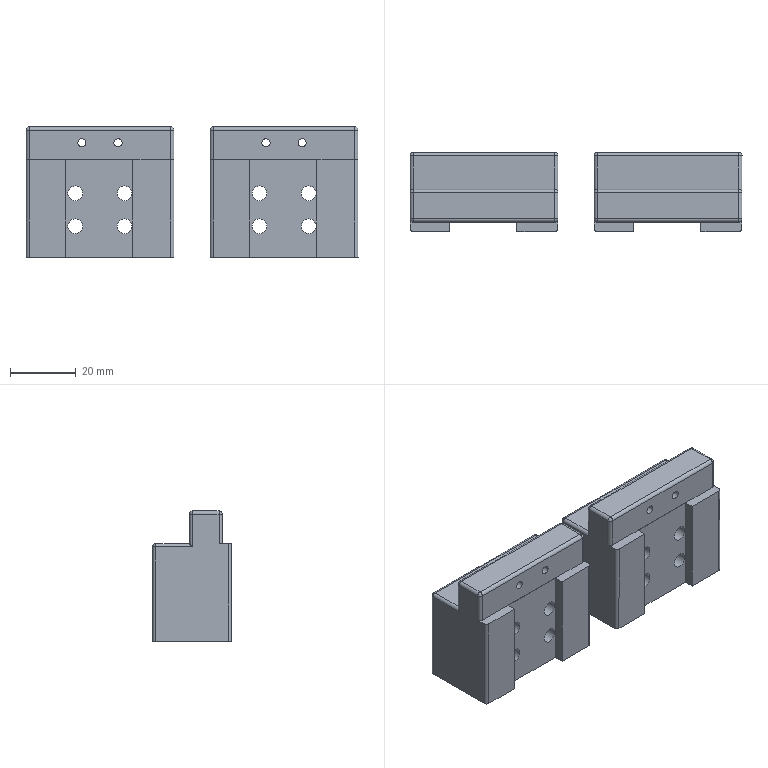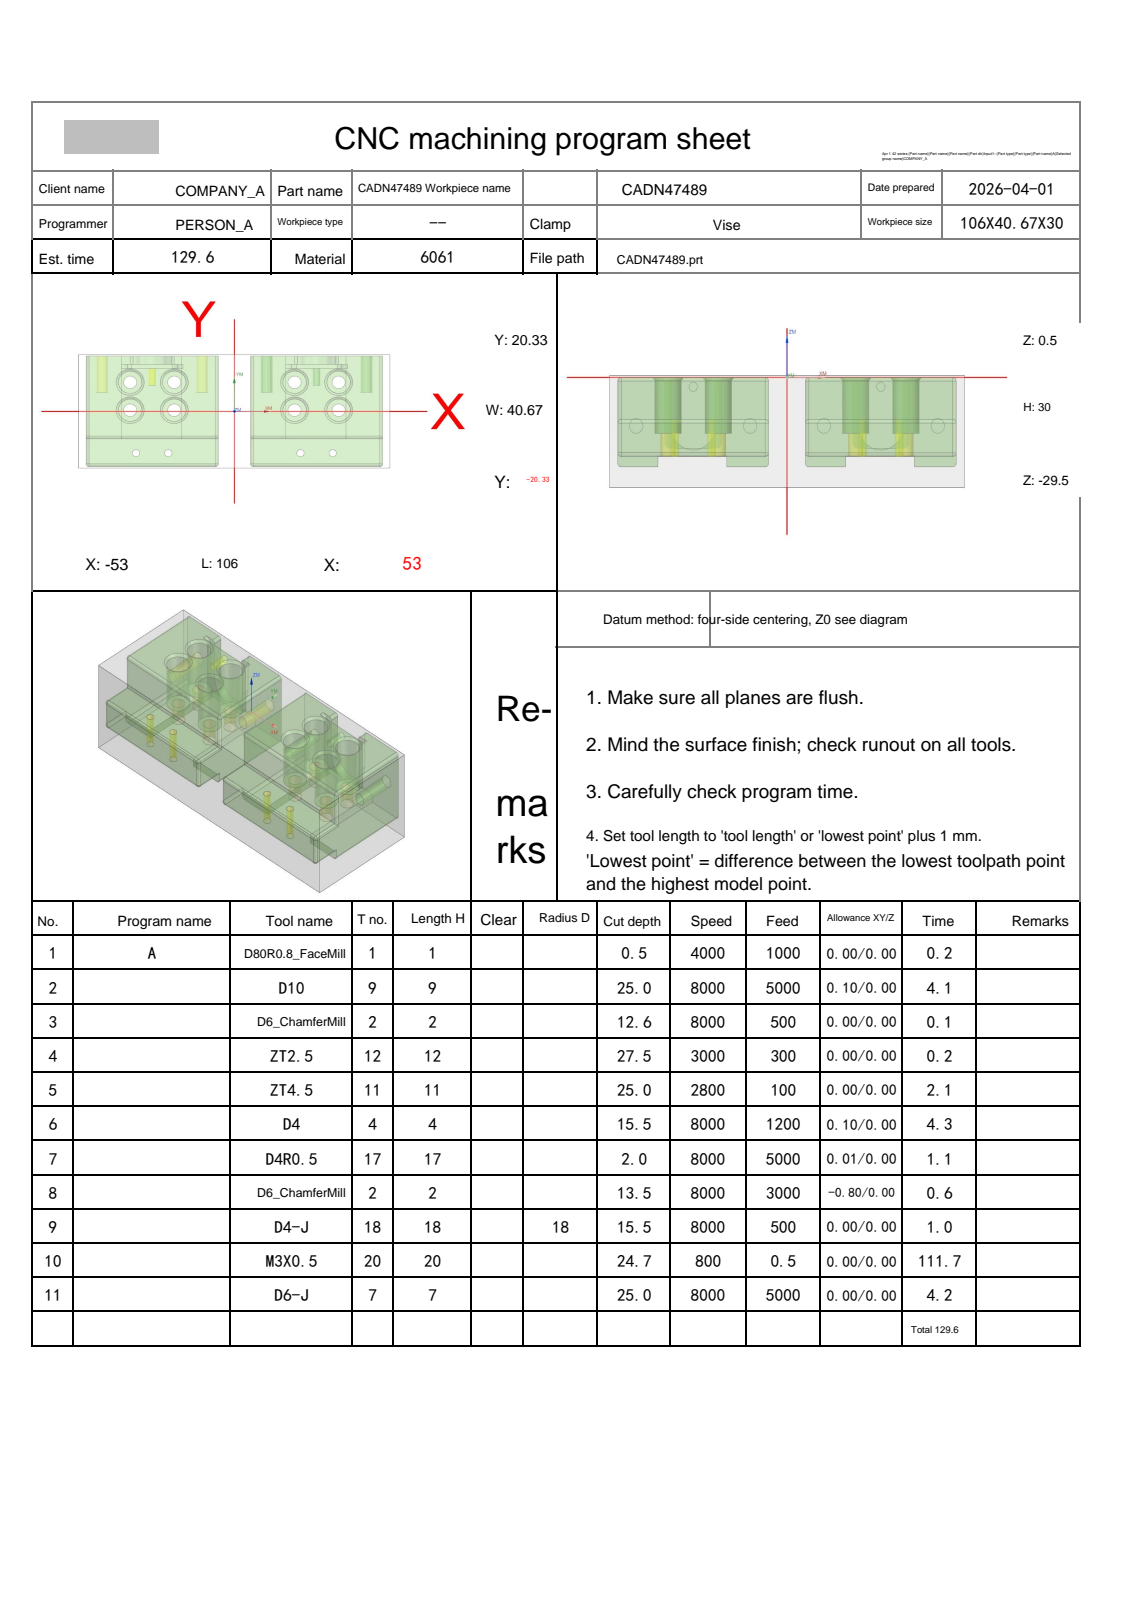NC program | NX | posted by the shop | part box 101.001 x 24.001 x 39.667 mm
Lines 23223 to 24072 of 28944:
N7 T17 M06
(D4R0.5  D=4. R=0.5 H=17 ce=0.01 di=0.00)
G00 G90 G54 X51.277 Y23.99 M03 S8000
G43 H17 Z10.5
M08
Z.478
G01 Z-.022 F5000.
X51.026 Y20.759
X51.176 Y19.806
X51.175 Y15.568
X51.22 Y-8.835
G02 X49.5 Y-10.554 I-1.72 J0.0
G01 X6.5
G02 X4.779 Y-8.833 I0.0 J1.721
G01 X4.785 Y19.806
X4.996 Y20.837
X4.879 Y20.846 Z-.029
X4.815 Y20.851 Z-.036
X4.676 Y19.806
X4.671 Y-8.833
G03 X6.5 Y-10.662 I1.829 J0.0
G01 X49.5
G03 X51.328 Y-8.834 I0.0 J1.828
G01 X51.3 Y19.806
X51.197 Y20.654
X51.196 Y20.858
X51.288 Y20.885 Z-.053
X51.401 Y19.806
Y-8.834
G02 X49.5 Y-10.735 I-1.901 J0.0
G01 X6.5
G02 X4.598 Y-8.833 I0.0 J1.902
G01 X4.618 Y-8.735
X4.612 Y19.806
X4.74 Y20.893
X4.657 Y20.931 Z-.076
X4.532 Y19.806
X4.523 Y-8.833
G03 X6.5 Y-10.81 I1.977 J0.0
G01 X49.5
G03 X51.476 Y-8.834 I0.0 J1.976
G01 X51.458 Y19.806
X51.369 Y20.92
X51.416 Y20.927 Z-.089
X51.442 Y20.931 Z-.103
X51.528 Y19.806
X51.553 Y-8.834
G02 X49.5 Y-10.887 I-2.053 J0.0
G01 X6.5
G02 X4.446 Y-8.833 I0.0 J2.054
G01 X4.466 Y19.806
X4.585 Y20.931
X4.531 Z-.12
X4.498 Z-.136
X4.386 Y19.806
X4.368 Y-8.833
G03 X6.5 Y-10.965 I2.132 J0.0
G01 X49.5 Y-10.966
G03 X51.632 Y-8.834 I0.0 J2.132
G01 X51.612 Y19.806
G02 X51.519 Y20.931 I10.05 J1.395
G01 X51.57 Z-.156
X51.609 Z-.175
G03 X51.701 Y19.806 I12.91 J.486
G01 X51.711 Y-8.834
G02 X49.5 Y-11.045 I-2.211 J0.0
G01 X6.5
G02 X4.288 Y-8.833 I0.0 J2.211
G01 X4.297 Y19.806
G03 X4.396 Y20.931 I-11.071 J1.537
G01 X4.343 Z-.198
X4.297 Z-.22
X4.215 Y19.806
X4.214 Y-8.735
X4.209 Y-8.833
G03 X6.5 Y-11.124 I2.291 J0.0
G01 X49.5 Y-11.125
G03 X51.79 Y-8.834 I0.0 J2.291
G01 X51.782 Y19.806
G02 X51.703 Y20.931 I9.664 J1.242
G01 X51.749 Z-.246
X51.787 Z-.272
G03 X51.859 Y19.806 I10.894 J.13
G01 X51.869 Y-8.834
G02 X49.5 Y-11.203 I-2.369 J0.0
G01 X6.5 Y-11.202
G02 X4.131 Y-8.833 I0.0 J2.369
G01 X4.137 Y-8.735
X4.144 Y19.806
G03 X4.21 Y20.931 I-10.878 J1.202
G01 X4.17 Z-.3
X4.133 Z-.329
G02 X4.067 Y19.806 I-11.04 J.081
G01 X4.062 Y-8.735
X4.054 Y-8.833
G03 X6.5 Y-11.279 I2.445 J0.0
G01 X49.5
G03 X51.945 Y-8.834 I0.0 J2.445
G01 X51.933 Y19.806
G02 X51.868 Y20.931 I10.58 J1.177
G01 X51.909 Z-.36
X51.949 Z-.391
G03 X52.008 Y19.806 I14.116 J.168
G01 X52.018 Y-8.834
G02 X49.5 Y-11.353 I-2.518 J0.0
G01 X6.5 Y-11.352
G02 X3.981 Y-8.833 I0.0 J2.519
G01 X3.986 Y-8.735
Y19.806
G03 X4.053 Y20.931 I-10.043 J1.159
G01 X4.011 Z-.425
X3.968 Z-.459
G02 X3.921 Y19.806 I-14.021 J.021
G01 X3.911 Y-8.833
G03 X6.5 Y-11.422 I2.589 J0.0
G01 X49.5 Y-11.423
G03 X52.088 Y-8.834 I0.0 J2.588
G01 X52.084 Y-8.735
X52.085 Y19.806
G02 X52.033 Y20.924 I12.009 J1.117
G01 Y20.931
X52.062 Z-.495
X52.096 Z-.531
Y20.929
G03 X52.146 Y19.806 I12.537 J0.0
G01 X52.148 Y-8.735
X52.154 Y-8.834
G02 X49.5 Y-11.488 I-2.654 J0.0
G01 X6.5 Y-11.487
G02 X3.846 Y-8.833 I0.0 J2.654
G01 X3.858 Y19.806
G03 X3.908 Y20.91 I-12.043 J1.104
G01 Y20.931
X3.874 Z-.57
X3.846 Z-.609
G02 X3.796 Y19.806 I-13.278 J.019
G01 X3.794 Y5.677
X3.789 Y-8.735
X3.784 Y-8.833
G03 X6.5 Y-11.549 I2.715 J0.0
G01 X49.5
G03 X52.215 Y-8.834 I0.0 J2.715
G01 X52.211 Y-8.735
X52.206 Y19.806
G02 X52.156 Y20.911 I12.214 J1.105
G01 Y20.931
X52.187 Z-.649
X52.218 Z-.69
G03 X52.266 Y19.806 I13.411 J.011
G01 X52.267 Y-8.735
X52.271 Y-8.834
G02 X49.5 Y-11.606 I-2.771 J0.0
G01 X49.412 Y-11.599
X6.656 Y-11.598
X6.5 Y-11.605
G02 X3.728 Y-8.833 I0.0 J2.772
G01 X3.738 Y19.806
G03 X3.783 Y20.826 I-11.463 J1.02
G01 X3.782 Y20.931
X3.755 Y20.932 Z-.732
X3.73 Z-.775
Y20.88
G02 X3.679 Y19.806 I-11.362 J0.0
G01 X3.677 Y-8.833
G03 X6.5 Y-11.656 I2.822 J0.0
G01 X6.656 Y-11.648
X49.412 Y-11.649
X49.5 Y-11.657
G03 X52.322 Y-8.834 I0.0 J2.822
G01 X52.314 Y-8.735
X52.321 Y-7.605
Y19.806
X52.308 Y20.089
X52.276 Y20.372
G02 X52.269 Y20.702 I7.382 J.33
X52.272 Y20.927 I7.39 J0.0
G01 X52.294 Z-.819
X52.318 Z-.864
G03 X52.311 Y20.686 I4.008 J-.241
X52.332 Y20.275 I4.015 J0.0
G02 X52.36 Y19.734 I-5.265 J-.543
G01 X52.368 Y-8.834
G02 X49.5 Y-11.702 I-2.868 J0.0
G01 X6.5 Y-11.701
G02 X3.632 Y-8.833 I0.0 J2.868
G01 X3.643 Y19.806
G03 X3.685 Y20.932 I-21.161 J1.356
G01 X3.664 Y20.933 Z-.909
X3.653 Z-.955
G02 X3.606 Y19.806 I-35.766 J.954
G01 X3.596 Y-8.735
X3.593 Y-8.833
G03 X6.5 Y-11.74 I2.907 J0.0
G01 X6.656 Y-11.734
X49.412 Y-11.735
X49.5 Y-11.741
G03 X52.407 Y-8.834 I0.0 J2.907
G01 X52.399 Y19.806
G02 X52.356 Y20.928 I19.168 J1.292
G01 X52.375 Z-1.002
X52.392 Z-1.049
G03 X52.438 Y19.806 I20.417 J.261
G01 X52.44 Y-8.834
G02 X49.5 Y-11.774 I-2.94 J0.0
G01 X49.412 Y-11.769
X6.5 Y-11.773
G02 X3.56 Y-8.833 I0.0 J2.94
G01 X3.567 Y19.806
G02 X3.6 Y20.372 I5.899 J-.06
G01 X3.607 Y20.932
X3.589 Y20.931 Z-1.097
X3.575 Z-1.145
G02 X3.578 Y20.726 I-7.299 J-.206
X3.541 Y19.991 I-7.302 J0.0
G01 X3.533 Y-8.833
G03 X6.5 Y-11.8 I2.967 J0.0
G01 X49.5 Y-11.801
G03 X52.467 Y-8.834 I0.0 J2.967
G01 X52.464 Y-8.735
Y19.806
X52.427 Y20.928
X52.44 Z-1.19
X52.453 Z-1.234
X52.485 Y19.806
X52.484 Y-8.735
X52.486 Y-8.834
G02 X49.5 Y-11.82 I-2.986 J0.0
G01 X49.412 Y-11.815
X18.548 Y-11.818
X18.265 Y-11.814
X6.656
X6.5 Y-11.819
G02 X3.514 Y-8.833 I0.0 J2.986
G01 X3.518 Y2.498
X3.524 Y3.699
Y19.806
G02 X3.557 Y20.372 I6.727 J-.108
G01 X3.561 Y20.931
X3.553 Z-1.278
X3.546 Z-1.323
X3.547 Y20.87
G02 X3.512 Y19.806 I-16.343 J0.0
G01 X3.506 Y-8.805
X3.501 Y-8.833
G03 X6.5 Y-11.832 I2.999 J0.0
G01 X6.656 Y-11.825
X49.412
X49.5 Y-11.833
G03 X52.499 Y-8.834 I0.0 J2.999
G01 X52.496 Y-8.735
X52.497 Y19.806
G02 X52.474 Y20.928 I55.865 J1.711
G01 X52.479 Z-1.367
X52.484 Z-1.411
X52.504 Y19.806
Y-8.735
X52.507 Y-8.834
G02 X49.5 Y-11.841 I-3.007 J0.0
G01 X49.412 Y-11.836
X6.939 Y-11.835
X6.5 Y-11.84
G02 X3.493 Y-8.833 I0.0 J3.007
G01 X3.5 Y19.714
G02 X3.534 Y20.372 I6.27 J-.002
G01 X3.532 Y20.928
X3.527 Z-1.5
X3.526 Y20.372
G03 X3.491 Y19.704 I6.246 J-.667
G01 X3.49 Y-8.858
G03 X6.489 Y-11.843 I3.011 J.026
G01 X49.497 Y-11.844
G03 X52.509 Y-8.831 I0.0 J3.013
G01 X52.51 Y19.806
G02 X52.489 Y20.866 I27.36 J1.06
G01 Y20.928
G00 Z10.5
X-4.78 Y24.019
Z.478
G01 Z-.022
X-4.958 Y20.778
X-4.783 Y19.806
X-4.788 Y-8.735
X-4.779 Y-8.834
G02 X-6.5 Y-10.555 I-1.721 J0.0
G01 X-49.5
G02 X-51.223 Y-8.832 I0.0 J1.723
G01 X-51.164 Y19.943
G02 X-51.021 Y20.795 I2.643 J-.005
G01 X-51.124 Y20.839 Z-.029
X-51.175 Y20.872 Z-.036
X-51.302 Y19.806
X-51.323 Y16.415
X-51.33 Y-8.832
G03 X-49.5 Y-10.662 I1.83 J0.0
G01 X-6.5 Y-10.663
G03 X-4.671 Y-8.833 I0.0 J1.829
G01 X-4.675 Y19.806
X-4.796 Y20.654
X-4.797 Y20.839
X-4.719 Y20.896 Z-.053
X-4.616 Y19.948
X-4.598 Y-8.833
G02 X-6.5 Y-10.735 I-1.902 J0.0
G01 X-49.5 Y-10.734
G02 X-51.402 Y-8.832 I0.0 J1.902
G01 X-51.401 Y19.806
X-51.272 Y20.892
X-51.346 Y20.917 Z-.076
X-51.458 Y19.806
X-51.469 Y-8.735
X-51.478 Y-8.832
G03 X-49.5 Y-10.81 I1.977 J0.0
G01 X-6.5
G03 X-4.523 Y-8.833 I0.0 J1.977
G01 X-4.538 Y19.948
X-4.574 Y20.089
X-4.636 Y20.931
X-4.591 Z-.089
X-4.552 Z-.103
Y20.84
G03 X-4.465 Y19.806 I6.172 J0.0
G01 Y-8.735
X-4.446 Y-8.833
G02 X-6.5 Y-10.887 I-2.054 J0.0
G01 X-49.5 Y-10.886
G02 X-51.554 Y-8.832 I0.0 J2.054
G01 X-51.528 Y19.806
X-51.425 Y20.932
X-51.47 Z-.12
X-51.507 Z-.136
X-51.612 Y19.806
X-51.633 Y-8.832
G03 X-49.5 Y-10.965 I2.133 J0.0
G01 X-6.5 Y-10.966
G03 X-4.368 Y-8.833 I0.0 J2.132
G01 X-4.387 Y19.922
G02 X-4.474 Y20.794 I4.339 J.872
G01 X-4.472 Y20.931
X-4.429 Z-.156
X-4.387 Z-.175
G03 X-4.296 Y19.806 I8.515 J.117
G01 X-4.289 Y-8.833
G02 X-6.5 Y-11.045 I-2.212 J0.0
G01 X-49.5 Y-11.044
G02 X-51.712 Y-8.832 I0.0 J2.212
G01 X-51.701 Y19.806
X-51.604 Y20.932
X-51.658 Z-.198
X-51.702 Z-.22
G02 X-51.783 Y19.806 I-9.803 J.135
G01 X-51.791 Y-8.832
G03 X-49.5 Y-11.123 I2.291 J0.0
G01 X-6.5 Y-11.124
G03 X-4.209 Y-8.833 I0.0 J2.291
G01 X-4.214 Y-8.735
Y19.806
G02 X-4.294 Y20.931 I13.107 J1.497
G01 X-4.251 Y20.932 Z-.246
X-4.209 Z-.272
G03 X-4.143 Y19.806 I10.99 J.077
G01 X-4.137 Y-8.735
X-4.131 Y-8.833
G02 X-6.5 Y-11.203 I-2.369 J0.0
G01 X-49.5 Y-11.202
G02 X-51.87 Y-8.832 I0.0 J2.37
G01 X-51.859 Y19.806
G03 X-51.788 Y20.932 I-11.095 J1.269
G01 X-51.83 Z-.3
X-51.868 Z-.329
G02 X-51.933 Y19.806 I-10.763 J.058
G01 X-51.946 Y-8.832
G03 X-49.5 Y-11.278 I2.446 J0.0
G01 X-6.5 Y-11.279
G03 X-4.055 Y-8.833 I0.0 J2.446
G01 X-4.062 Y-8.735
X-4.067 Y19.806
G02 X-4.132 Y20.932 I11.017 J1.208
G01 X-4.091 Z-.36
X-4.052 Z-.391
G03 X-3.986 Y19.806 I10.088 J.032
G01 Y-8.735
X-3.981 Y-8.833
G02 X-6.5 Y-11.352 I-2.519 J0.0
G01 X-49.5 Y-11.351
G02 X-52.019 Y-8.832 I0.0 J2.519
G01 X-52.008 Y19.806
G03 X-51.949 Y20.932 I-12.162 J1.195
G01 X-51.989 Z-.425
X-52.032 Z-.459
Y20.865
G02 X-52.085 Y19.806 I-10.535 J0.0
G01 Y-8.735
X-52.089 Y-8.832
G03 X-49.5 Y-11.421 I2.589 J0.0
G01 X-6.5 Y-11.422
G03 X-3.911 Y-8.833 I0.0 J2.589
G01 X-3.92 Y19.806
G02 X-3.967 Y20.932 I14.303 J1.169
G01 X-3.937 Z-.495
X-3.907 Z-.531
Y20.912
G03 X-3.857 Y19.806 I12.216 J0.0
G01 X-3.846 Y-8.833
G02 X-6.5 Y-11.488 I-2.654 J0.0
G01 X-49.5 Y-11.487
G02 X-52.155 Y-8.832 I0.0 J2.655
G01 X-52.148 Y-8.735
X-52.146 Y19.806
G03 X-52.096 Y20.929 I-12.592 J1.123
G01 Y20.932
X-52.126 Z-.57
X-52.156 Z-.609
Y20.917
G02 X-52.205 Y19.806 I-12.391 J0.0
G01 X-52.211 Y-8.735
X-52.216 Y-8.832
G03 X-49.5 Y-11.548 I2.716 J0.0
G01 X-6.5 Y-11.549
G03 X-3.785 Y-8.833 I0.0 J2.716
G01 X-3.796 Y19.806
G02 X-3.845 Y20.932 I13.3 J1.147
G01 X-3.813 Z-.649
X-3.782 Z-.69
Y20.828
G03 X-3.737 Y19.806 I11.672 J0.0
G01 X-3.728 Y-8.833
G02 X-6.5 Y-11.605 I-2.772 J0.0
G01 X-6.653 Y-11.598
X-49.409 Y-11.597
X-49.5 Y-11.604
G02 X-52.272 Y-8.832 I0.0 J2.772
G01 X-52.27 Y-8.735
X-52.266 Y19.839
G03 X-52.218 Y20.886 I-11.351 J1.047
G01 Y20.932
X-52.249 Y20.929 Z-.732
X-52.272 Y20.927 Z-.775
X-52.27 Y20.787
G02 X-52.317 Y19.945 I-7.655 J0.0
G01 X-52.323 Y-8.832
G03 X-49.5 Y-11.655 I2.823 J0.0
G01 X-49.409 Y-11.647
X-6.653 Y-11.648
X-6.5 Y-11.656
G03 X-3.678 Y-8.833 I0.0 J2.823
G01 Y-8.735
Y19.806
G02 X-3.728 Y20.849 I10.765 J1.043
G01 Y20.932
X-3.706 Z-.819
X-3.682 Z-.864
G03 X-3.642 Y19.806 I16.882 J.041
G01 X-3.632 Y-8.833
G02 X-6.5 Y-11.701 I-2.868 J0.0
G01 X-49.5 Y-11.7
G02 X-52.368 Y-8.832 I0.0 J2.868
G01 X-52.359 Y19.84
G03 X-52.316 Y20.908 I-13.048 J1.068
G01 Y20.927
X-52.347 Z-.955
X-52.355 Y20.918
Y20.877
G02 X-52.398 Y19.84 I-12.525 J0.0
G01 X-52.407 Y-8.832
G03 X-49.5 Y-11.739 I2.907 J0.0
G01 X-49.409 Y-11.733
X-6.653 Y-11.734
X-6.5 Y-11.74
G03 X-3.593 Y-8.833 I0.0 J2.907
G01 X-3.605 Y19.806
G02 X-3.644 Y20.932 I22.211 J1.323
G01 X-3.625 Z-1.002
X-3.606 Z-1.049
G03 X-3.568 Y19.806 I21.512 J.163
G01 X-3.56 Y-8.833
G02 X-6.5 Y-11.773 I-2.94 J0.0
G01 X-6.653 Y-11.768
X-49.5 Y-11.772
G02 X-52.44 Y-8.832 I0.0 J2.94
G01 X-52.437 Y19.841
G03 X-52.393 Y20.879 I-12.287 J1.038
G01 Y20.927
X-52.411 Z-1.097
X-52.421 Y20.928 Z-1.145
Y20.843
G02 X-52.461 Y19.841 I-12.391 J0.0
G01 X-52.467 Y-8.832
G03 X-49.5 Y-11.799 I2.967 J0.0
G01 X-6.5 Y-11.8
G03 X-3.533 Y-8.833 I0.0 J2.967
G01 X-3.534 Y-8.735
X-3.533 Y19.806
G02 X-3.574 Y20.932 I24.977 J1.464
G01 X-3.557 Z-1.19
X-3.545 Z-1.234
X-3.515 Y19.806
X-3.516 Y-8.735
X-3.514 Y-8.833
G02 X-6.5 Y-11.819 I-2.986 J0.0
G01 X-6.653 Y-11.814
X-49.5 Y-11.818
G02 X-52.486 Y-8.832 I0.0 J2.986
G01 X-52.479 Y19.841
G03 X-52.439 Y20.788 I-11.322 J.947
G01 X-52.44 Y20.928
X-52.447 Z-1.278
X-52.454 Z-1.323
X-52.453 Y20.77
G02 X-52.49 Y19.841 I-11.589 J0.0
G01 X-52.492 Y-8.735
X-52.499 Y-8.832
G03 X-49.5 Y-11.831 I2.999 J0.0
G01 X-49.409 Y-11.824
X-49.126
X-6.653 Y-11.825
X-6.5 Y-11.833
G03 X-3.501 Y-8.833 I0.0 J2.999
G01 X-3.506 Y-8.735
Y19.806
X-3.528 Y20.928
X-3.521 Z-1.367
X-3.516 Z-1.411
X-3.497 Y19.806
X-3.498 Y-8.735
X-3.493 Y-8.833
G02 X-6.5 Y-11.841 I-3.007 J0.0
G01 X-6.653 Y-11.835
X-23.359 Y-11.834
X-23.642 Y-11.835
X-49.409 Y-11.836
X-49.5 Y-11.839
G02 X-52.507 Y-8.832 I0.0 J3.007
G01 X-52.502 Y-8.735
X-52.501 Y19.842
G03 X-52.466 Y20.73 I-11.115 J.889
G01 X-52.468 Y20.928
X-52.472 Z-1.5
X-52.471 Y20.823
G02 X-52.509 Y19.824 I-13.154 J0.0
G01 X-52.51 Y-8.876
G03 X-49.5 Y-11.842 I3.011 J.046
G01 X-6.5 Y-11.843
G03 X-3.49 Y-8.876 I0.0 J3.01
G01 Y-8.833
Y19.806
X-3.515 Y20.928
G00 Z10.5
G91 G28 Z0.0
M05
M09
G91 G28 Z0.0
M01
N8 T02 M06
(D6_ChamferMill  D=6. R=0. H=02 ce=0.00 di=0.00)
G00 G90 G54 X-20.749 Y21.96 M03 S8000
G43 H02 Z20.
M08
Z2.085
G01 Z-1.501 F3000.
G03 X-20.83 Y21.66 I.52 J-.3
X-20.53 Y21.14 I.6 J0.0
G01 X-20.5 Y21.132
X-6.5
X-6.47 Y21.14
G03 X-6.17 Y21.659 I-.3 J.52
X-6.25 Y21.959 I-.6 J0.0
G01 Z2.085
G00 Z20.
X-49.749 Y21.96
Z2.085
G01 Z-1.501
G03 X-49.83 Y21.66 I.52 J-.3
X-49.53 Y21.141 I.6 J0.0
G01 X-49.5 Y21.132
X-35.5
X-35.47 Y21.14
G03 X-35.17 Y21.66 I-.3 J.52
X-35.25 Y21.96 I-.6 J0.0
G01 Z2.085
G00 Z20.
X35.251 Y21.959
Z2.084
G01 Z-1.501
G03 X35.17 Y21.659 I.52 J-.3
X35.47 Y21.139 I.6 J0.0
G01 X35.5 Y21.131
X49.5
X49.53 Y21.139
G03 X49.83 Y21.659 I-.3 J.52
X49.75 Y21.959 I-.6 J0.0
G01 Z2.084
G00 Z20.
X6.251
Z2.085
G01 Z-1.501
G03 X6.17 Y21.659 I.52 J-.3
X6.47 Y21.14 I.6 J0.0
G01 X6.5 Y21.132
X20.5 Y21.131
X20.53 Y21.139
G03 X20.83 Y21.659 I-.3 J.52
X20.75 Y21.959 I-.6 J0.0
G01 Z2.085
G00 Z20.
G00 G90 X33.5 Y-14.983 M03 S8000
Z20.
G98 G81 X33.5 Y-14.983 Z-13.009 R-8.259 F500.
X22.5
X-22.5 Y-14.982
X-33.5
G80
G00 Z20.
G00 G90 X-33.239 Y-1.555 M03 S8000
Z20.
Z.699
G01 X-33.19 Y-1.503 Z.673 F500.
X-32.968 Y-1.199 Z.536
X-32.834 Y-.967 Z.439
X-32.682 Y-.623 Z.302
X-32.574 Y-.262 Z.165
X-32.512 Y.109 Z.028
X-32.497 Y.485 Z-.109
X-32.529 Y.859 Z-.246
X-32.607 Y1.227 Z-.383
X-32.731 Y1.583 Z-.52
X-32.899 Y1.919 Z-.657
X-33.107 Y2.233 Z-.794
X-33.352 Y2.518 Z-.931
X-33.632 Y2.77 Z-1.068
X-33.94 Y2.985 Z-1.204
X-34.273 Y3.159 Z-1.341
X-34.626 Y3.291 Z-1.478
X-34.992 Y3.378 Z-1.615
X-35.366 Y3.418 Z-1.752
X-35.5 Z-1.801
G03 X-38.501 Y.418 I0.0 J-3.001
X-35.5 Y-2.583 I3.001 J0.0
X-32.499 Y.418 I0.0 J3.001
X-35.5 Y3.418 I-3.001 J0.0
X-35.998 Y3.377 I0.0 J-3.001
G01 Z.699
G00 Z20.
X-33.239 Y8.445
Z.699
G01 X-33.19 Y8.497 Z.673
X-32.968 Y8.801 Z.536
X-32.834 Y9.033 Z.439
X-32.682 Y9.377 Z.302
X-32.574 Y9.738 Z.165
X-32.512 Y10.109 Z.028
X-32.497 Y10.485 Z-.109
X-32.529 Y10.859 Z-.246
X-32.607 Y11.227 Z-.383
X-32.731 Y11.583 Z-.52
X-32.898 Y11.919 Z-.657
X-33.107 Y12.233 Z-.794
X-33.352 Y12.518 Z-.931
X-33.632 Y12.77 Z-1.068
X-33.94 Y12.985 Z-1.204
X-34.273 Y13.159 Z-1.341
X-34.626 Y13.291 Z-1.478
X-34.992 Y13.378 Z-1.615
X-35.366 Y13.418 Z-1.752
X-35.5 Z-1.801
G03 X-38.501 Y10.418 I0.0 J-3.001
X-35.5 Y7.417 I3.001 J0.0
X-32.499 Y10.418 I0.0 J3.001
X-35.5 Y13.418 I-3.001 J0.0
X-35.997 Y13.377 I0.0 J-3.001
G01 Z.699
G00 Z20.
X-18.239 Y8.445
Z.699
G01 X-18.19 Y8.497 Z.673
X-17.968 Y8.801 Z.536
X-17.834 Y9.033 Z.439
X-17.682 Y9.377 Z.302
X-17.574 Y9.738 Z.165
X-17.512 Y10.109 Z.028
X-17.497 Y10.484 Z-.109
X-17.529 Y10.859 Z-.246
X-17.607 Y11.227 Z-.383
X-17.731 Y11.582 Z-.52
X-17.898 Y11.919 Z-.657
X-18.107 Y12.233 Z-.794
X-18.352 Y12.517 Z-.931
X-18.632 Y12.769 Z-1.068
X-18.94 Y12.984 Z-1.204
X-19.273 Y13.159 Z-1.341
X-19.626 Y13.291 Z-1.478
X-19.992 Y13.378 Z-1.615
X-20.366 Y13.418 Z-1.752
X-20.5 Z-1.801
G03 X-23.501 Y10.417 I0.0 J-3.001
X-20.5 Y7.417 I3.001 J0.0
X-17.499 Y10.417 I0.0 J3.001
X-20.5 Y13.418 I-3.001 J0.0
X-20.997 Y13.376 I0.0 J-3.001
G01 Z.699
G00 Z20.
X-18.239 Y-1.555
Z.699
G01 X-18.19 Y-1.503 Z.673
X-17.968 Y-1.199 Z.536
X-17.834 Y-.967 Z.439
X-17.682 Y-.623 Z.302
X-17.574 Y-.262 Z.165
X-17.512 Y.109 Z.028
X-17.497 Y.484 Z-.109
X-17.529 Y.859 Z-.246
X-17.607 Y1.227 Z-.383
X-17.731 Y1.582 Z-.52
X-17.899 Y1.919 Z-.657
X-18.107 Y2.233 Z-.794
X-18.352 Y2.517 Z-.931
X-18.632 Y2.769 Z-1.068
X-18.94 Y2.984 Z-1.204
X-19.273 Y3.159 Z-1.341
X-19.626 Y3.291 Z-1.478
X-19.992 Y3.378 Z-1.615
X-20.366 Y3.418 Z-1.752
X-20.5 Z-1.801
G03 X-23.501 Y.417 I0.0 J-3.001
X-20.5 Y-2.583 I3.001 J0.0
X-17.499 Y.417 I0.0 J3.001
X-20.5 Y3.418 I-3.001 J0.0
X-20.998 Y3.376 I0.0 J-3.001
G01 Z.699
G00 Z20.
X22.761 Y-1.556
Z.699
G01 X22.81 Y-1.504 Z.673
X23.032 Y-1.2 Z.536
X23.166 Y-.968 Z.439
X23.318 Y-.623 Z.302
X23.426 Y-.263 Z.165
X23.488 Y.108 Z.028
X23.503 Y.484 Z-.109
X23.471 Y.859 Z-.246
X23.393 Y1.226 Z-.383
X23.269 Y1.582 Z-.52
X23.101 Y1.918 Z-.657
X22.893 Y2.232 Z-.794
X22.648 Y2.517 Z-.931
X22.368 Y2.769 Z-1.068
X22.06 Y2.984 Z-1.204
X21.727 Y3.159 Z-1.341
X21.374 Y3.29 Z-1.478
X21.008 Y3.377 Z-1.615
X20.634 Y3.417 Z-1.752
X20.5 Z-1.801
G03 X17.499 Y.417 I0.0 J-3.001
X20.5 Y-2.584 I3.001 J0.0
X23.501 Y.417 I0.0 J3.001
X20.5 Y3.417 I-3.001 J0.0
X20.002 Y3.376 I0.0 J-3.001
G01 Z.699
G00 Z20.
X22.761 Y8.444
Z.699
G01 X22.81 Y8.496 Z.673
X23.032 Y8.8 Z.536
X23.166 Y9.032 Z.439
X23.318 Y9.377 Z.302
X23.426 Y9.737 Z.165
X23.488 Y10.108 Z.028
X23.503 Y10.484 Z-.109
X23.471 Y10.859 Z-.246
X23.393 Y11.226 Z-.383
X23.269 Y11.582 Z-.52
X23.102 Y11.918 Z-.657
X22.893 Y12.232 Z-.794
X22.648 Y12.517 Z-.931
X22.368 Y12.769 Z-1.068
X22.06 Y12.984 Z-1.204
X21.727 Y13.159 Z-1.341
X21.374 Y13.29 Z-1.478
X21.008 Y13.377 Z-1.615
X20.634 Y13.417 Z-1.752
X20.5 Z-1.801
G03 X17.499 Y10.417 I0.0 J-3.001
X20.5 Y7.416 I3.001 J0.0
X23.501 Y10.417 I0.0 J3.001
X20.5 Y13.417 I-3.001 J0.0
X20.003 Y13.376 I0.0 J-3.001
G01 Z.699
G00 Z20.
X37.761 Y8.444
Z.699
G01 X37.81 Y8.496 Z.673
X38.032 Y8.8 Z.536
X38.166 Y9.032 Z.439
X38.318 Y9.376 Z.302
X38.426 Y9.737 Z.165
X38.488 Y10.108 Z.028
X38.503 Y10.484 Z-.109
X38.471 Y10.858 Z-.246
X38.393 Y11.226 Z-.383
X38.269 Y11.581 Z-.52
X38.102 Y11.918 Z-.657
X37.893 Y12.232 Z-.794
X37.648 Y12.516 Z-.931
X37.368 Y12.768 Z-1.068
X37.06 Y12.983 Z-1.204
X36.727 Y13.158 Z-1.341
X36.374 Y13.29 Z-1.478
X36.008 Y13.377 Z-1.615
X35.634 Y13.417 Z-1.752
X35.5 Z-1.801
G03 X32.499 Y10.416 I0.0 J-3.001
X35.5 Y7.416 I3.001 J0.0
X38.501 Y10.416 I0.0 J3.001
X35.5 Y13.417 I-3.001 J0.0
X35.003 Y13.376 I0.0 J-3.001
G01 Z.699
G00 Z20.
X37.761 Y-1.556
Z.699
G01 X37.81 Y-1.504 Z.673
X38.032 Y-1.2 Z.536
X38.166 Y-.968 Z.439
X38.318 Y-.624 Z.302
X38.426 Y-.263 Z.165
X38.488 Y.108 Z.028
X38.503 Y.484 Z-.109
X38.471 Y.858 Z-.246
X38.393 Y1.226 Z-.383
X38.269 Y1.581 Z-.52
X38.101 Y1.918 Z-.657
X37.893 Y2.232 Z-.794
X37.648 Y2.516 Z-.931
X37.368 Y2.768 Z-1.068
X37.06 Y2.983 Z-1.204
X36.727 Y3.158 Z-1.341
X36.374 Y3.29 Z-1.478
X36.008 Y3.377 Z-1.615
X35.634 Y3.417 Z-1.752
X35.5 Z-1.801
G03 X32.499 Y.416 I0.0 J-3.001
X35.5 Y-2.584 I3.001 J0.0
X38.501 Y.416 I0.0 J3.001
X35.5 Y3.417 I-3.001 J0.0
X35.002 Y3.376 I0.0 J-3.001
G01 Z.699
G00 Z20.
G91 G28 Z0.0
M05
M09
G91 G28 Z0.0
M01